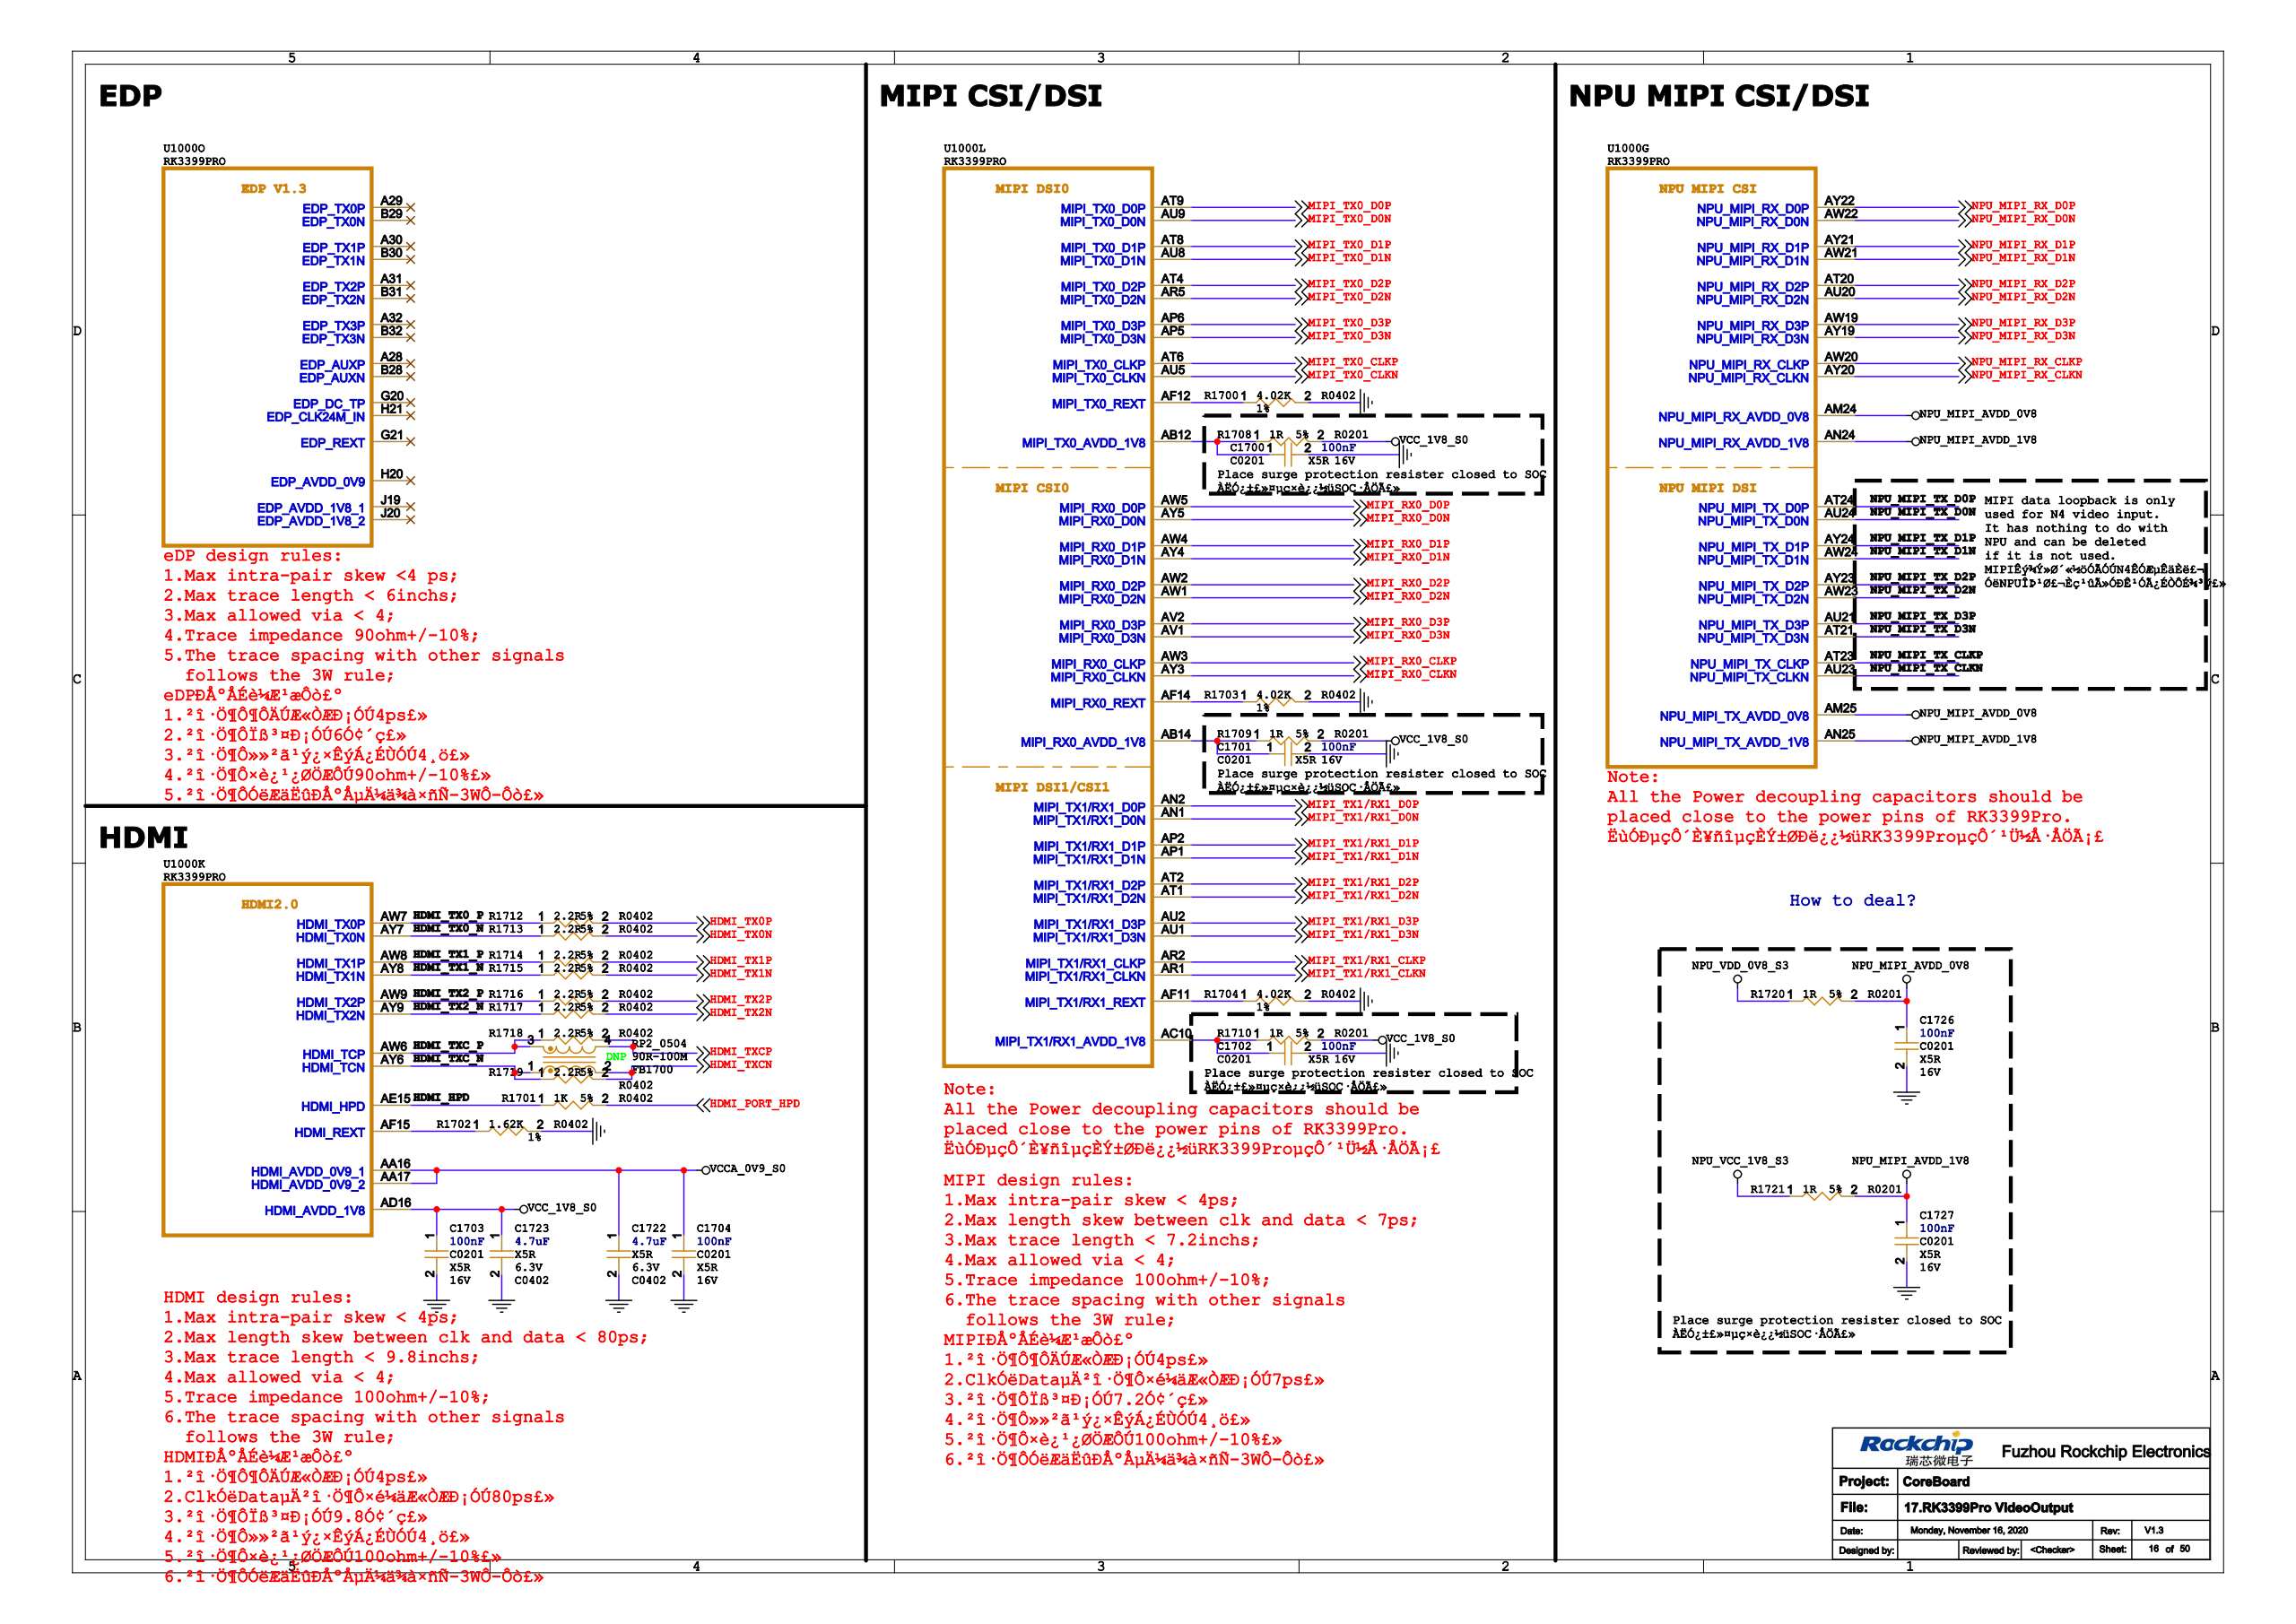Circuit board | Cadence Allegro | 749 parts | 717 nets | one sheet of the schematic
Parts on this sheet (reference | value | footprint):
C1700 | 100nF | C0201
C1701 | 100nF | C0201
C1702 | 100nF | C0201
C1703 | 100nF | C0201
C1704 | 100nF | C0201
C1722 | 4.7uF | C0402
C1723 | 4.7uF | C0402
C1726 | 100nF | C0201
C1727 | 100nF | C0201
FB1700 | 90R-100M | RP2_0504
R1700 | 4.02K | R0402
R1702 | 1.62K | R0402
R1703 | 4.02K | R0402
R1704 | 4.02K | R0402
R1712 | 2.2R | R0402
R1713 | 2.2R | R0402
R1714 | 2.2R | R0402
R1715 | 2.2R | R0402
R1716 | 2.2R | R0402
R1717 | 2.2R | R0402
R1718 | 2.2R | R0402
R1719 | 2.2R | R0402
U1000 | RK3399PRO | BGA1372_27R00X27R00X2R19
Nets of these parts (net: part-pin ...):
GND: C1700-2 C1701-2 C1702-2 C1703-2 C1704-2 C1722-2 C1723-2 C1726-2 C1727-2 R1700-2 R1702-2 R1703-2 R1704-2
MIPI_TX0_D0P: U1000-AT9
HDMI_TX1N: R1715-2
MIPI_TX0_CLKP: U1000-AT6
HDMI_TX0P: R1712-2
MIPI_TX0_CLKN: U1000-AU5
HDMI_TX0N: R1713-2
MIPI_TX0_D2P: U1000-AT4
HDMI_TX2P: R1716-2
HDMI_TXCP: FB1700-4 R1718-2
MIPI_TX0_D2N: U1000-AR5
HDMI_TXCN: FB1700-2 R1719-2
MIPI_TX0_D3P: U1000-AP6
MIPI_RX0_D0N: U1000-AY5
MIPI_TX0_D3N: U1000-AP5
MIPI_RX0_D0P: U1000-AW5
MIPI_TX0_D0N: U1000-AU9
MIPI_RX0_D1N: U1000-AY4
MIPI_RX0_D1P: U1000-AW4
MIPI_RX0_CLKN: U1000-AY3
HDMI_TX2N: R1717-2
MIPI_RX0_CLKP: U1000-AW3
MIPI_RX0_D2N: U1000-AW1
MIPI_RX0_D2P: U1000-AW2
MIPI_RX0_D3N: U1000-AV1
MIPI_RX0_D3P: U1000-AV2
MIPI_TX0_D1P: U1000-AT8
VCC_1V8_S0: C1703-1 C1723-1 U1000-AD16
HDMI_TX1P: R1714-2
MIPI_TX0_D1N: U1000-AU8
MIPI_TX1/RX1_D0N: U1000-AN1
MIPI_TX1/RX1_D0P: U1000-AN2
MIPI_TX1/RX1_D1N: U1000-AP1
MIPI_TX1/RX1_D1P: U1000-AP2
MIPI_TX1/RX1_CLKN: U1000-AR1
MIPI_TX1/RX1_CLKP: U1000-AR2
MIPI_TX1/RX1_D2N: U1000-AT1
MIPI_TX1/RX1_D2P: U1000-AT2
MIPI_TX1/RX1_D3N: U1000-AU1
MIPI_TX1/RX1_D3P: U1000-AU2
HDMI_TXC_N: FB1700-1 R1719-1 U1000-AY6
HDMI_TXC_P: FB1700-3 R1718-1 U1000-AW6
HDMI_HPD: U1000-AE15
HDMI_TX0_P: R1712-1 U1000-AW7
HDMI_TX0_N: R1713-1 U1000-AY7
HDMI_TX1_P: R1714-1 U1000-AW8
HDMI_TX1_N: R1715-1 U1000-AY8
HDMI_TX2_P: R1716-1 U1000-AW9
HDMI_TX2_N: R1717-1 U1000-AY9
VCCA_0V9_S0: C1704-1 C1722-1 U1000-AA16 U1000-AA17
N82631585: R1702-1 U1000-AF15
N82629264: C1701-1 U1000-AB14
N82628852: R1703-1 U1000-AF14
N82629419: C1700-1 U1000-AB12
N78542743: R1700-1 U1000-AF12
N82629100: C1702-1 U1000-AC10
N82628519: R1704-1 U1000-AF11
NPU_MIPI_AVDD_0V8: C1726-1 U1000-AM24 U1000-AM25
NPU_MIPI_RX_CLKN: U1000-AY20
NPU_MIPI_RX_CLKP: U1000-AW20
NPU_MIPI_RX_D0N: U1000-AW22
NPU_MIPI_RX_D1N: U1000-AW21
NPU_MIPI_RX_D2N: U1000-AU20
NPU_MIPI_RX_D3N: U1000-AY19
NPU_MIPI_RX_D0P: U1000-AY22
NPU_MIPI_RX_D1P: U1000-AY21
NPU_MIPI_RX_D2P: U1000-AT20
NPU_MIPI_RX_D3P: U1000-AW19
NPU_MIPI_TX_CLKN: U1000-AU23
NPU_MIPI_TX_CLKP: U1000-AT23
NPU_MIPI_TX_D0N: U1000-AU24
NPU_MIPI_TX_D1N: U1000-AW24
NPU_MIPI_TX_D2N: U1000-AW23
NPU_MIPI_TX_D3N: U1000-AT21
NPU_MIPI_TX_D0P: U1000-AT24
NPU_MIPI_TX_D1P: U1000-AY24
NPU_MIPI_TX_D2P: U1000-AY23
NPU_MIPI_TX_D3P: U1000-AU21
NPU_MIPI_AVDD_1V8: C1727-1 U1000-AN24 U1000-AN25